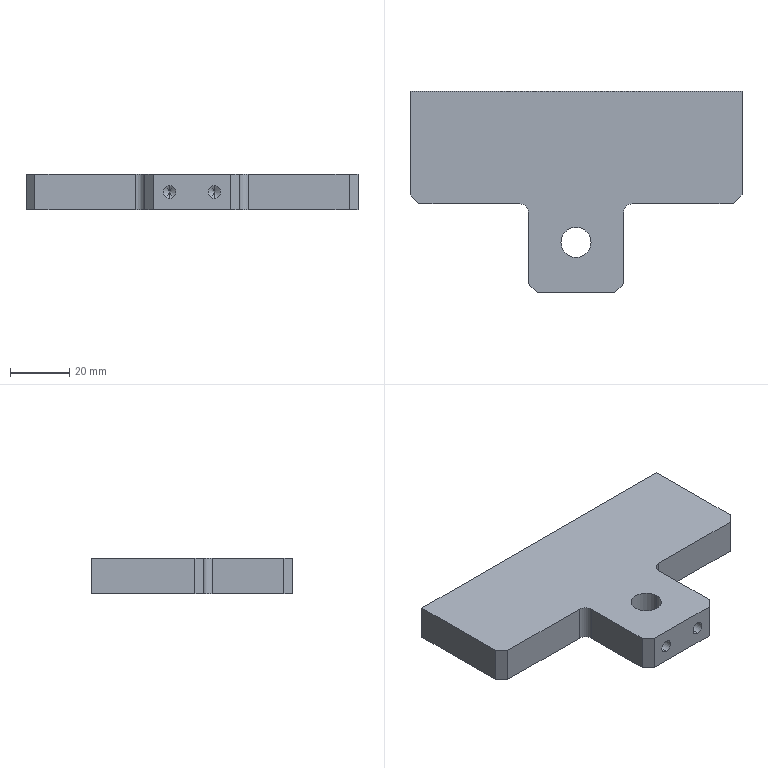Part | SolidWorks | features HoleWzd 3, Chamfer 1, Cut 1, Extrusion 1, Fillet 1, MirrorPattern 1 | 1 solid | 38 faces | box 112 x 68 x 12 mm | volume 60173 mm3 | cylinder 14 | plane 14 | cone 10 | commonest cylinder face diameters 5 x6 4.2 x4 6 x2 10.2 x2
STEP:
#1=CARTESIAN_POINT('',(63.5,12.4,8.1));
#2=VERTEX_POINT('',#1);
#3=CARTESIAN_POINT('',(63.5,12.4,3.9));
#4=VERTEX_POINT('',#3);
#5=CARTESIAN_POINT('',(63.5,12.4,6.));
#6=DIRECTION('',(0.,-1.,0.));
#7=DIRECTION('',(0.,0.,-1.));
#8=AXIS2_PLACEMENT_3D('',#5,#6,#7);
#9=CIRCLE('',#8,2.1);
#10=EDGE_CURVE('',#2,#4,#9,.T.);
#11=ORIENTED_EDGE('',*,*,#10,.F.);
#12=CARTESIAN_POINT('',(63.5,0.,8.1));
#13=VERTEX_POINT('',#12);
#14=CARTESIAN_POINT('',(63.5,0.,8.1));
#15=DIRECTION('',(0.,-1.,0.));
#16=VECTOR('',#15,1000.);
#17=LINE('',#14,#16);
#18=EDGE_CURVE('',#2,#13,#17,.T.);
#19=ORIENTED_EDGE('',*,*,#18,.T.);
#20=CARTESIAN_POINT('',(63.5,0.,3.9));
#21=VERTEX_POINT('',#20);
#22=CARTESIAN_POINT('',(63.5,0.,6.));
#23=DIRECTION('',(0.,-1.,0.));
#24=DIRECTION('',(0.,0.,-1.));
#25=AXIS2_PLACEMENT_3D('',#22,#23,#24);
#26=CIRCLE('',#25,2.1);
#27=EDGE_CURVE('',#13,#21,#26,.T.);
#28=ORIENTED_EDGE('',*,*,#27,.T.);
#29=CARTESIAN_POINT('',(63.5,0.,3.9));
#30=DIRECTION('',(0.,-1.,0.));
#31=VECTOR('',#30,1000.);
#32=LINE('',#29,#31);
#33=EDGE_CURVE('',#4,#21,#32,.T.);
#34=ORIENTED_EDGE('',*,*,#33,.F.);
#35=EDGE_LOOP('',(#11,#19,#28,#34));
#36=FACE_OUTER_BOUND('',#35,.T.);
#37=CARTESIAN_POINT('',(63.5,0.,6.));
#38=DIRECTION('',(0.,-1.,0.));
#39=DIRECTION('',(0.,0.,-1.));
#40=AXIS2_PLACEMENT_3D('',#37,#38,#39);
#41=CYLINDRICAL_SURFACE('',#40,2.1);
#42=ADVANCED_FACE('',(#36),#41,.F.);
#43=CARTESIAN_POINT('',(63.5,13.662,6.));
#44=VERTEX_POINT('',#43);
#45=CARTESIAN_POINT('',(63.5,12.4,3.9));
#46=DIRECTION('',(0.,-0.515,-0.8572));
#47=VECTOR('',#46,1000.);
#48=LINE('',#45,#47);
#49=EDGE_CURVE('',#44,#4,#48,.T.);
#50=ORIENTED_EDGE('',*,*,#49,.F.);
#51=CARTESIAN_POINT('',(63.5,12.4,8.1));
#52=DIRECTION('',(0.,-0.515,0.8572));
#53=VECTOR('',#52,1000.);
#54=LINE('',#51,#53);
#55=EDGE_CURVE('',#44,#2,#54,.T.);
#56=ORIENTED_EDGE('',*,*,#55,.T.);
#57=ORIENTED_EDGE('',*,*,#10,.T.);
#58=EDGE_LOOP('',(#50,#56,#57));
#59=FACE_OUTER_BOUND('',#58,.T.);
#60=CARTESIAN_POINT('',(63.5,12.4,6.));
#61=DIRECTION('',(0.,-1.,0.));
#62=DIRECTION('',(0.,0.,-1.));
#63=AXIS2_PLACEMENT_3D('',#60,#61,#62);
#64=CONICAL_SURFACE('',#63,2.1,1.03);
#65=ADVANCED_FACE('',(#59),#64,.F.);
#66=CARTESIAN_POINT('',(48.5,12.4,8.1));
#67=VERTEX_POINT('',#66);
#68=CARTESIAN_POINT('',(48.5,12.4,3.9));
#69=VERTEX_POINT('',#68);
#70=CARTESIAN_POINT('',(48.5,12.4,6.));
#71=DIRECTION('',(0.,-1.,0.));
#72=DIRECTION('',(0.,0.,-1.));
#73=AXIS2_PLACEMENT_3D('',#70,#71,#72);
#74=CIRCLE('',#73,2.1);
#75=EDGE_CURVE('',#67,#69,#74,.T.);
#76=ORIENTED_EDGE('',*,*,#75,.F.);
#77=CARTESIAN_POINT('',(48.5,0.,8.1));
#78=VERTEX_POINT('',#77);
#79=CARTESIAN_POINT('',(48.5,0.,8.1));
#80=DIRECTION('',(0.,-1.,0.));
#81=VECTOR('',#80,1000.);
#82=LINE('',#79,#81);
#83=EDGE_CURVE('',#67,#78,#82,.T.);
#84=ORIENTED_EDGE('',*,*,#83,.T.);
#85=CARTESIAN_POINT('',(48.5,0.,3.9));
#86=VERTEX_POINT('',#85);
#87=CARTESIAN_POINT('',(48.5,0.,6.));
#88=DIRECTION('',(0.,-1.,0.));
#89=DIRECTION('',(0.,0.,-1.));
#90=AXIS2_PLACEMENT_3D('',#87,#88,#89);
#91=CIRCLE('',#90,2.1);
#92=EDGE_CURVE('',#78,#86,#91,.T.);
#93=ORIENTED_EDGE('',*,*,#92,.T.);
#94=CARTESIAN_POINT('',(48.5,0.,3.9));
#95=DIRECTION('',(0.,-1.,0.));
#96=VECTOR('',#95,1000.);
#97=LINE('',#94,#96);
#98=EDGE_CURVE('',#69,#86,#97,.T.);
#99=ORIENTED_EDGE('',*,*,#98,.F.);
#100=EDGE_LOOP('',(#76,#84,#93,#99));
#101=FACE_OUTER_BOUND('',#100,.T.);
#102=CARTESIAN_POINT('',(48.5,0.,6.));
#103=DIRECTION('',(0.,-1.,0.));
#104=DIRECTION('',(0.,0.,-1.));
#105=AXIS2_PLACEMENT_3D('',#102,#103,#104);
#106=CYLINDRICAL_SURFACE('',#105,2.1);
#107=ADVANCED_FACE('',(#101),#106,.F.);
#108=CARTESIAN_POINT('',(48.5,13.662,6.));
#109=VERTEX_POINT('',#108);
#110=CARTESIAN_POINT('',(48.5,12.4,3.9));
#111=DIRECTION('',(0.,-0.515,-0.8572));
#112=VECTOR('',#111,1000.);
#113=LINE('',#110,#112);
#114=EDGE_CURVE('',#109,#69,#113,.T.);
#115=ORIENTED_EDGE('',*,*,#114,.F.);
#116=CARTESIAN_POINT('',(48.5,12.4,8.1));
#117=DIRECTION('',(0.,-0.515,0.8572));
#118=VECTOR('',#117,1000.);
#119=LINE('',#116,#118);
#120=EDGE_CURVE('',#109,#67,#119,.T.);
#121=ORIENTED_EDGE('',*,*,#120,.T.);
#122=ORIENTED_EDGE('',*,*,#75,.T.);
#123=EDGE_LOOP('',(#115,#121,#122));
#124=FACE_OUTER_BOUND('',#123,.T.);
#125=CARTESIAN_POINT('',(48.5,12.4,6.));
#126=DIRECTION('',(0.,-1.,0.));
#127=DIRECTION('',(0.,0.,-1.));
#128=AXIS2_PLACEMENT_3D('',#125,#126,#127);
#129=CONICAL_SURFACE('',#128,2.1,1.03);
#130=ADVANCED_FACE('',(#124),#129,.F.);
#131=CARTESIAN_POINT('',(101.,53.,3.5));
#132=VERTEX_POINT('',#131);
#133=CARTESIAN_POINT('',(101.,53.,8.5));
#134=VERTEX_POINT('',#133);
#135=CARTESIAN_POINT('',(101.,53.,6.));
#136=DIRECTION('',(0.,1.,0.));
#137=DIRECTION('',(0.,0.,1.));
#138=AXIS2_PLACEMENT_3D('',#135,#136,#137);
#139=CIRCLE('',#138,2.5);
#140=EDGE_CURVE('',#132,#134,#139,.T.);
#141=ORIENTED_EDGE('',*,*,#140,.F.);
#142=CARTESIAN_POINT('',(101.,68.,3.5));
#143=VERTEX_POINT('',#142);
#144=CARTESIAN_POINT('',(101.,68.,3.5));
#145=DIRECTION('',(0.,1.,0.));
#146=VECTOR('',#145,1000.);
#147=LINE('',#144,#146);
#148=EDGE_CURVE('',#132,#143,#147,.T.);
#149=ORIENTED_EDGE('',*,*,#148,.T.);
#150=CARTESIAN_POINT('',(101.,68.,8.5));
#151=VERTEX_POINT('',#150);
#152=CARTESIAN_POINT('',(101.,68.,6.));
#153=DIRECTION('',(0.,1.,0.));
#154=DIRECTION('',(0.,0.,1.));
#155=AXIS2_PLACEMENT_3D('',#152,#153,#154);
#156=CIRCLE('',#155,2.5);
#157=EDGE_CURVE('',#143,#151,#156,.T.);
#158=ORIENTED_EDGE('',*,*,#157,.T.);
#159=CARTESIAN_POINT('',(101.,68.,8.5));
#160=DIRECTION('',(0.,1.,0.));
#161=VECTOR('',#160,1000.);
#162=LINE('',#159,#161);
#163=EDGE_CURVE('',#134,#151,#162,.T.);
#164=ORIENTED_EDGE('',*,*,#163,.F.);
#165=EDGE_LOOP('',(#141,#149,#158,#164));
#166=FACE_OUTER_BOUND('',#165,.T.);
#167=CARTESIAN_POINT('',(101.,68.,6.));
#168=DIRECTION('',(0.,1.,0.));
#169=DIRECTION('',(0.,0.,1.));
#170=AXIS2_PLACEMENT_3D('',#167,#168,#169);
#171=CYLINDRICAL_SURFACE('',#170,2.5);
#172=ADVANCED_FACE('',(#166),#171,.F.);
#173=CARTESIAN_POINT('',(101.,51.498,6.));
#174=VERTEX_POINT('',#173);
#175=CARTESIAN_POINT('',(101.,53.,8.5));
#176=DIRECTION('',(0.,0.515,0.8572));
#177=VECTOR('',#176,1000.);
#178=LINE('',#175,#177);
#179=EDGE_CURVE('',#174,#134,#178,.T.);
#180=ORIENTED_EDGE('',*,*,#179,.F.);
#181=CARTESIAN_POINT('',(101.,53.,3.5));
#182=DIRECTION('',(0.,0.515,-0.8572));
#183=VECTOR('',#182,1000.);
#184=LINE('',#181,#183);
#185=EDGE_CURVE('',#174,#132,#184,.T.);
#186=ORIENTED_EDGE('',*,*,#185,.T.);
#187=ORIENTED_EDGE('',*,*,#140,.T.);
#188=EDGE_LOOP('',(#180,#186,#187));
#189=FACE_OUTER_BOUND('',#188,.T.);
#190=CARTESIAN_POINT('',(101.,53.,6.));
#191=DIRECTION('',(0.,1.,0.));
#192=DIRECTION('',(0.,0.,1.));
#193=AXIS2_PLACEMENT_3D('',#190,#191,#192);
#194=CONICAL_SURFACE('',#193,2.5,1.03);
#195=ADVANCED_FACE('',(#189),#194,.F.);
#196=CARTESIAN_POINT('',(56.,53.,3.5));
#197=VERTEX_POINT('',#196);
#198=CARTESIAN_POINT('',(56.,53.,8.5));
#199=VERTEX_POINT('',#198);
#200=CARTESIAN_POINT('',(56.,53.,6.));
#201=DIRECTION('',(0.,1.,0.));
#202=DIRECTION('',(0.,0.,1.));
#203=AXIS2_PLACEMENT_3D('',#200,#201,#202);
#204=CIRCLE('',#203,2.5);
#205=EDGE_CURVE('',#197,#199,#204,.T.);
#206=ORIENTED_EDGE('',*,*,#205,.F.);
#207=CARTESIAN_POINT('',(56.,68.,3.5));
#208=VERTEX_POINT('',#207);
#209=CARTESIAN_POINT('',(56.,68.,3.5));
#210=DIRECTION('',(0.,1.,0.));
#211=VECTOR('',#210,1000.);
#212=LINE('',#209,#211);
#213=EDGE_CURVE('',#197,#208,#212,.T.);
#214=ORIENTED_EDGE('',*,*,#213,.T.);
#215=CARTESIAN_POINT('',(56.,68.,8.5));
#216=VERTEX_POINT('',#215);
#217=CARTESIAN_POINT('',(56.,68.,6.));
#218=DIRECTION('',(0.,1.,0.));
#219=DIRECTION('',(0.,0.,1.));
#220=AXIS2_PLACEMENT_3D('',#217,#218,#219);
#221=CIRCLE('',#220,2.5);
#222=EDGE_CURVE('',#208,#216,#221,.T.);
#223=ORIENTED_EDGE('',*,*,#222,.T.);
#224=CARTESIAN_POINT('',(56.,68.,8.5));
#225=DIRECTION('',(0.,1.,0.));
#226=VECTOR('',#225,1000.);
#227=LINE('',#224,#226);
#228=EDGE_CURVE('',#199,#216,#227,.T.);
#229=ORIENTED_EDGE('',*,*,#228,.F.);
#230=EDGE_LOOP('',(#206,#214,#223,#229));
#231=FACE_OUTER_BOUND('',#230,.T.);
#232=CARTESIAN_POINT('',(56.,68.,6.));
#233=DIRECTION('',(0.,1.,0.));
#234=DIRECTION('',(0.,0.,1.));
#235=AXIS2_PLACEMENT_3D('',#232,#233,#234);
#236=CYLINDRICAL_SURFACE('',#235,2.5);
#237=ADVANCED_FACE('',(#231),#236,.F.);
#238=CARTESIAN_POINT('',(56.,51.498,6.));
#239=VERTEX_POINT('',#238);
#240=CARTESIAN_POINT('',(56.,53.,8.5));
#241=DIRECTION('',(0.,0.515,0.8572));
#242=VECTOR('',#241,1000.);
#243=LINE('',#240,#242);
#244=EDGE_CURVE('',#239,#199,#243,.T.);
#245=ORIENTED_EDGE('',*,*,#244,.F.);
#246=CARTESIAN_POINT('',(56.,53.,3.5));
#247=DIRECTION('',(0.,0.515,-0.8572));
#248=VECTOR('',#247,1000.);
#249=LINE('',#246,#248);
#250=EDGE_CURVE('',#239,#197,#249,.T.);
#251=ORIENTED_EDGE('',*,*,#250,.T.);
#252=ORIENTED_EDGE('',*,*,#205,.T.);
#253=EDGE_LOOP('',(#245,#251,#252));
#254=FACE_OUTER_BOUND('',#253,.T.);
#255=CARTESIAN_POINT('',(56.,53.,6.));
#256=DIRECTION('',(0.,1.,0.));
#257=DIRECTION('',(0.,0.,1.));
#258=AXIS2_PLACEMENT_3D('',#255,#256,#257);
#259=CONICAL_SURFACE('',#258,2.5,1.03);
#260=ADVANCED_FACE('',(#254),#259,.F.);
#261=CARTESIAN_POINT('',(11.,53.,3.5));
#262=VERTEX_POINT('',#261);
#263=CARTESIAN_POINT('',(11.,53.,8.5));
#264=VERTEX_POINT('',#263);
#265=CARTESIAN_POINT('',(11.,53.,6.));
#266=DIRECTION('',(0.,1.,0.));
#267=DIRECTION('',(0.,0.,1.));
#268=AXIS2_PLACEMENT_3D('',#265,#266,#267);
#269=CIRCLE('',#268,2.5);
#270=EDGE_CURVE('',#262,#264,#269,.T.);
#271=ORIENTED_EDGE('',*,*,#270,.F.);
#272=CARTESIAN_POINT('',(11.,68.,3.5));
#273=VERTEX_POINT('',#272);
#274=CARTESIAN_POINT('',(11.,68.,3.5));
#275=DIRECTION('',(0.,1.,0.));
#276=VECTOR('',#275,1000.);
#277=LINE('',#274,#276);
#278=EDGE_CURVE('',#262,#273,#277,.T.);
#279=ORIENTED_EDGE('',*,*,#278,.T.);
#280=CARTESIAN_POINT('',(11.,68.,8.5));
#281=VERTEX_POINT('',#280);
#282=CARTESIAN_POINT('',(11.,68.,6.));
#283=DIRECTION('',(0.,1.,0.));
#284=DIRECTION('',(0.,0.,1.));
#285=AXIS2_PLACEMENT_3D('',#282,#283,#284);
#286=CIRCLE('',#285,2.5);
#287=EDGE_CURVE('',#273,#281,#286,.T.);
#288=ORIENTED_EDGE('',*,*,#287,.T.);
#289=CARTESIAN_POINT('',(11.,68.,8.5));
#290=DIRECTION('',(0.,1.,0.));
#291=VECTOR('',#290,1000.);
#292=LINE('',#289,#291);
#293=EDGE_CURVE('',#264,#281,#292,.T.);
#294=ORIENTED_EDGE('',*,*,#293,.F.);
#295=EDGE_LOOP('',(#271,#279,#288,#294));
#296=FACE_OUTER_BOUND('',#295,.T.);
#297=CARTESIAN_POINT('',(11.,68.,6.));
#298=DIRECTION('',(0.,1.,0.));
#299=DIRECTION('',(0.,0.,1.));
#300=AXIS2_PLACEMENT_3D('',#297,#298,#299);
#301=CYLINDRICAL_SURFACE('',#300,2.5);
#302=ADVANCED_FACE('',(#296),#301,.F.);
#303=CARTESIAN_POINT('',(11.,51.498,6.));
#304=VERTEX_POINT('',#303);
#305=CARTESIAN_POINT('',(11.,53.,8.5));
#306=DIRECTION('',(0.,0.515,0.8572));
#307=VECTOR('',#306,1000.);
#308=LINE('',#305,#307);
#309=EDGE_CURVE('',#304,#264,#308,.T.);
#310=ORIENTED_EDGE('',*,*,#309,.F.);
#311=CARTESIAN_POINT('',(11.,53.,3.5));
#312=DIRECTION('',(0.,0.515,-0.8572));
#313=VECTOR('',#312,1000.);
#314=LINE('',#311,#313);
#315=EDGE_CURVE('',#304,#262,#314,.T.);
#316=ORIENTED_EDGE('',*,*,#315,.T.);
#317=ORIENTED_EDGE('',*,*,#270,.T.);
#318=EDGE_LOOP('',(#310,#316,#317));
#319=FACE_OUTER_BOUND('',#318,.T.);
#320=CARTESIAN_POINT('',(11.,53.,6.));
#321=DIRECTION('',(0.,1.,0.));
#322=DIRECTION('',(0.,0.,1.));
#323=AXIS2_PLACEMENT_3D('',#320,#321,#322);
#324=CONICAL_SURFACE('',#323,2.5,1.03);
#325=ADVANCED_FACE('',(#319),#324,.F.);
#326=CARTESIAN_POINT('',(50.9,17.,0.));
#327=VERTEX_POINT('',#326);
#328=CARTESIAN_POINT('',(61.1,17.,0.));
#329=VERTEX_POINT('',#328);
#330=CARTESIAN_POINT('',(56.,17.,0.));
#331=DIRECTION('',(0.,0.,1.));
#332=DIRECTION('',(1.,0.,0.));
#333=AXIS2_PLACEMENT_3D('',#330,#331,#332);
#334=CIRCLE('',#333,5.1);
#335=EDGE_CURVE('',#327,#329,#334,.T.);
#336=ORIENTED_EDGE('',*,*,#335,.F.);
#337=CARTESIAN_POINT('',(50.9,17.,12.));
#338=VERTEX_POINT('',#337);
#339=CARTESIAN_POINT('',(50.9,17.,12.));
#340=DIRECTION('',(0.,0.,1.));
#341=VECTOR('',#340,1000.);
#342=LINE('',#339,#341);
#343=EDGE_CURVE('',#327,#338,#342,.T.);
#344=ORIENTED_EDGE('',*,*,#343,.T.);
#345=CARTESIAN_POINT('',(61.1,17.,12.));
#346=VERTEX_POINT('',#345);
#347=CARTESIAN_POINT('',(56.,17.,12.));
#348=DIRECTION('',(0.,0.,1.));
#349=DIRECTION('',(1.,0.,0.));
#350=AXIS2_PLACEMENT_3D('',#347,#348,#349);
#351=CIRCLE('',#350,5.1);
#352=EDGE_CURVE('',#338,#346,#351,.T.);
#353=ORIENTED_EDGE('',*,*,#352,.T.);
#354=CARTESIAN_POINT('',(61.1,17.,12.));
#355=DIRECTION('',(0.,0.,1.));
#356=VECTOR('',#355,1000.);
#357=LINE('',#354,#356);
#358=EDGE_CURVE('',#329,#346,#357,.T.);
#359=ORIENTED_EDGE('',*,*,#358,.F.);
#360=EDGE_LOOP('',(#336,#344,#353,#359));
#361=FACE_OUTER_BOUND('',#360,.T.);
#362=CARTESIAN_POINT('',(56.,17.,12.));
#363=DIRECTION('',(0.,0.,1.));
#364=DIRECTION('',(1.,0.,0.));
#365=AXIS2_PLACEMENT_3D('',#362,#363,#364);
#366=CYLINDRICAL_SURFACE('',#365,5.1);
#367=ADVANCED_FACE('',(#361),#366,.F.);
#368=CARTESIAN_POINT('',(63.5,0.,6.));
#369=DIRECTION('',(0.,-1.,0.));
#370=DIRECTION('',(0.,0.,-1.));
#371=AXIS2_PLACEMENT_3D('',#368,#369,#370);
#372=CIRCLE('',#371,2.1);
#373=EDGE_CURVE('',#21,#13,#372,.T.);
#374=ORIENTED_EDGE('',*,*,#373,.F.);
#375=ORIENTED_EDGE('',*,*,#27,.F.);
#376=EDGE_LOOP('',(#374,#375));
#377=FACE_BOUND('',#376,.T.);
#378=CARTESIAN_POINT('',(48.5,0.,6.));
#379=DIRECTION('',(0.,-1.,0.));
#380=DIRECTION('',(0.,0.,-1.));
#381=AXIS2_PLACEMENT_3D('',#378,#379,#380);
#382=CIRCLE('',#381,2.1);
#383=EDGE_CURVE('',#86,#78,#382,.T.);
#384=ORIENTED_EDGE('',*,*,#383,.F.);
#385=ORIENTED_EDGE('',*,*,#92,.F.);
#386=EDGE_LOOP('',(#384,#385));
#387=FACE_BOUND('',#386,.T.);
#388=CARTESIAN_POINT('',(43.,0.,0.));
#389=VERTEX_POINT('',#388);
#390=CARTESIAN_POINT('',(69.,0.,0.));
#391=VERTEX_POINT('',#390);
#392=CARTESIAN_POINT('',(0.,0.,0.));
#393=DIRECTION('',(1.,0.,0.));
#394=VECTOR('',#393,1000.);
#395=LINE('',#392,#394);
#396=EDGE_CURVE('',#389,#391,#395,.T.);
#397=ORIENTED_EDGE('',*,*,#396,.T.);
#398=CARTESIAN_POINT('',(69.,0.,12.));
#399=VERTEX_POINT('',#398);
#400=CARTESIAN_POINT('',(69.,0.,12.));
#401=DIRECTION('',(0.,0.,1.));
#402=VECTOR('',#401,1000.);
#403=LINE('',#400,#402);
#404=EDGE_CURVE('',#391,#399,#403,.T.);
#405=ORIENTED_EDGE('',*,*,#404,.T.);
#406=CARTESIAN_POINT('',(43.,0.,12.));
#407=VERTEX_POINT('',#406);
#408=CARTESIAN_POINT('',(0.,0.,12.));
#409=DIRECTION('',(1.,0.,0.));
#410=VECTOR('',#409,1000.);
#411=LINE('',#408,#410);
#412=EDGE_CURVE('',#407,#399,#411,.T.);
#413=ORIENTED_EDGE('',*,*,#412,.F.);
#414=CARTESIAN_POINT('',(43.,0.,12.));
#415=DIRECTION('',(0.,0.,-1.));
#416=VECTOR('',#415,1000.);
#417=LINE('',#414,#416);
#418=EDGE_CURVE('',#407,#389,#417,.T.);
#419=ORIENTED_EDGE('',*,*,#418,.T.);
#420=EDGE_LOOP('',(#397,#405,#413,#419));
#421=FACE_OUTER_BOUND('',#420,.T.);
#422=CARTESIAN_POINT('',(0.,0.,12.));
#423=DIRECTION('',(0.,1.,0.));
#424=DIRECTION('',(0.,0.,1.));
#425=AXIS2_PLACEMENT_3D('',#422,#423,#424);
#426=PLANE('',#425);
#427=ADVANCED_FACE('',(#377,#387,#421),#426,.F.);
#428=CARTESIAN_POINT('',(112.,33.,12.));
#429=VERTEX_POINT('',#428);
#430=CARTESIAN_POINT('',(112.,68.,12.));
#431=VERTEX_POINT('',#430);
#432=CARTESIAN_POINT('',(112.,0.,12.));
#433=DIRECTION('',(0.,1.,0.));
#434=VECTOR('',#433,1000.);
#435=LINE('',#432,#434);
#436=EDGE_CURVE('',#429,#431,#435,.T.);
#437=ORIENTED_EDGE('',*,*,#436,.F.);
#438=CARTESIAN_POINT('',(112.,33.,0.));
#439=VERTEX_POINT('',#438);
#440=CARTESIAN_POINT('',(112.,33.,0.));
#441=DIRECTION('',(0.,0.,-1.));
#442=VECTOR('',#441,1000.);
#443=LINE('',#440,#442);
#444=EDGE_CURVE('',#429,#439,#443,.T.);
#445=ORIENTED_EDGE('',*,*,#444,.T.);
#446=CARTESIAN_POINT('',(112.,68.,0.));
#447=VERTEX_POINT('',#446);
#448=CARTESIAN_POINT('',(112.,0.,0.));
#449=DIRECTION('',(0.,1.,0.));
#450=VECTOR('',#449,1000.);
#451=LINE('',#448,#450);
#452=EDGE_CURVE('',#439,#447,#451,.T.);
#453=ORIENTED_EDGE('',*,*,#452,.T.);
#454=CARTESIAN_POINT('',(112.,68.,12.));
#455=DIRECTION('',(0.,0.,-1.));
#456=VECTOR('',#455,1000.);
#457=LINE('',#454,#456);
#458=EDGE_CURVE('',#431,#447,#457,.T.);
#459=ORIENTED_EDGE('',*,*,#458,.F.);
#460=EDGE_LOOP('',(#437,#445,#453,#459));
#461=FACE_OUTER_BOUND('',#460,.T.);
#462=CARTESIAN_POINT('',(112.,0.,12.));
#463=DIRECTION('',(-1.,0.,0.));
#464=DIRECTION('',(0.,-1.,0.));
#465=AXIS2_PLACEMENT_3D('',#462,#463,#464);
#466=PLANE('',#465);
#467=ADVANCED_FACE('',(#461),#466,.F.);
#468=CARTESIAN_POINT('',(56.,17.,12.));
#469=DIRECTION('',(0.,0.,1.));
#470=DIRECTION('',(1.,0.,0.));
#471=AXIS2_PLACEMENT_3D('',#468,#469,#470);
#472=CIRCLE('',#471,5.1);
#473=EDGE_CURVE('',#346,#338,#472,.T.);
#474=ORIENTED_EDGE('',*,*,#473,.F.);
#475=ORIENTED_EDGE('',*,*,#352,.F.);
#476=EDGE_LOOP('',(#474,#475));
#477=FACE_BOUND('',#476,.T.);
#478=ORIENTED_EDGE('',*,*,#412,.T.);
#479=CARTESIAN_POINT('',(72.,3.,12.));
#480=VERTEX_POINT('',#479);
#481=CARTESIAN_POINT('',(69.,0.,12.));
#482=DIRECTION('',(0.7071,0.7071,0.));
#483=VECTOR('',#482,1000.);
#484=LINE('',#481,#483);
#485=EDGE_CURVE('',#399,#480,#484,.T.);
#486=ORIENTED_EDGE('',*,*,#485,.T.);
#487=CARTESIAN_POINT('',(72.,27.,12.));
#488=VERTEX_POINT('',#487);
#489=CARTESIAN_POINT('',(72.,0.,12.));
#490=DIRECTION('',(0.,1.,0.));
#491=VECTOR('',#490,1000.);
#492=LINE('',#489,#491);
#493=EDGE_CURVE('',#480,#488,#492,.T.);
#494=ORIENTED_EDGE('',*,*,#493,.T.);
#495=CARTESIAN_POINT('',(75.,30.,12.));
#496=VERTEX_POINT('',#495);
#497=CARTESIAN_POINT('',(75.,27.,12.));
#498=DIRECTION('',(0.,0.,-1.));
#499=DIRECTION('',(-1.,0.,0.));
#500=AXIS2_PLACEMENT_3D('',#497,#498,#499);
#501=CIRCLE('',#500,3.);
#502=EDGE_CURVE('',#488,#496,#501,.T.);
#503=ORIENTED_EDGE('',*,*,#502,.T.);
#504=CARTESIAN_POINT('',(109.,30.,12.));
#505=VERTEX_POINT('',#504);
#506=CARTESIAN_POINT('',(112.,30.,12.));
#507=DIRECTION('',(1.,0.,0.));
#508=VECTOR('',#507,1000.);
#509=LINE('',#506,#508);
#510=EDGE_CURVE('',#496,#505,#509,.T.);
#511=ORIENTED_EDGE('',*,*,#510,.T.);
#512=CARTESIAN_POINT('',(109.,30.,12.));
#513=DIRECTION('',(0.7071,0.7071,0.));
#514=VECTOR('',#513,1000.);
#515=LINE('',#512,#514);
#516=EDGE_CURVE('',#505,#429,#515,.T.);
#517=ORIENTED_EDGE('',*,*,#516,.T.);
#518=ORIENTED_EDGE('',*,*,#436,.T.);
#519=CARTESIAN_POINT('',(0.,68.,12.));
#520=VERTEX_POINT('',#519);
#521=CARTESIAN_POINT('',(0.,68.,12.));
#522=DIRECTION('',(-1.,0.,0.));
#523=VECTOR('',#522,1000.);
#524=LINE('',#521,#523);
#525=EDGE_CURVE('',#431,#520,#524,.T.);
#526=ORIENTED_EDGE('',*,*,#525,.T.);
#527=CARTESIAN_POINT('',(0.,33.,12.));
#528=VERTEX_POINT('',#527);
#529=CARTESIAN_POINT('',(0.,0.,12.));
#530=DIRECTION('',(0.,-1.,0.));
#531=VECTOR('',#530,1000.);
#532=LINE('',#529,#531);
#533=EDGE_CURVE('',#520,#528,#532,.T.);
#534=ORIENTED_EDGE('',*,*,#533,.T.);
#535=CARTESIAN_POINT('',(3.,30.,12.));
#536=VERTEX_POINT('',#535);
#537=CARTESIAN_POINT('',(0.,33.,12.));
#538=DIRECTION('',(0.7071,-0.7071,0.));
#539=VECTOR('',#538,1000.);
#540=LINE('',#537,#539);
#541=EDGE_CURVE('',#528,#536,#540,.T.);
#542=ORIENTED_EDGE('',*,*,#541,.T.);
#543=CARTESIAN_POINT('',(37.,30.,12.));
#544=VERTEX_POINT('',#543);
#545=CARTESIAN_POINT('',(0.,30.,12.));
#546=DIRECTION('',(-1.,0.,0.));
#547=VECTOR('',#546,1000.);
#548=LINE('',#545,#547);
#549=EDGE_CURVE('',#544,#536,#548,.T.);
#550=ORIENTED_EDGE('',*,*,#549,.F.);
#551=CARTESIAN_POINT('',(40.,27.,12.));
#552=VERTEX_POINT('',#551);
#553=CARTESIAN_POINT('',(37.,27.,12.));
#554=DIRECTION('',(0.,0.,-1.));
#555=DIRECTION('',(-1.,0.,0.));
#556=AXIS2_PLACEMENT_3D('',#553,#554,#555);
#557=CIRCLE('',#556,3.);
#558=EDGE_CURVE('',#544,#552,#557,.T.);
#559=ORIENTED_EDGE('',*,*,#558,.T.);
#560=CARTESIAN_POINT('',(40.,3.,12.));
#561=VERTEX_POINT('',#560);
#562=CARTESIAN_POINT('',(40.,0.,12.));
#563=DIRECTION('',(0.,1.,0.));
#564=VECTOR('',#563,1000.);
#565=LINE('',#562,#564);
#566=EDGE_CURVE('',#561,#552,#565,.T.);
#567=ORIENTED_EDGE('',*,*,#566,.F.);
#568=CARTESIAN_POINT('',(40.,3.,12.));
#569=DIRECTION('',(0.7071,-0.7071,0.));
#570=VECTOR('',#569,1000.);
#571=LINE('',#568,#570);
#572=EDGE_CURVE('',#561,#407,#571,.T.);
#573=ORIENTED_EDGE('',*,*,#572,.T.);
#574=EDGE_LOOP('',(#478,#486,#494,#503,#511,#517,#518,#526,#534,#542,#550,#559,#567,#573));
#575=FACE_OUTER_BOUND('',#574,.T.);
#576=CARTESIAN_POINT('',(0.,0.,12.));
#577=DIRECTION('',(0.,0.,-1.));
#578=DIRECTION('',(-1.,0.,0.));
#579=AXIS2_PLACEMENT_3D('',#576,#577,#578);
#580=PLANE('',#579);
#581=ADVANCED_FACE('',(#477,#575),#580,.F.);
#582=CARTESIAN_POINT('',(56.,17.,0.));
#583=DIRECTION('',(0.,0.,1.));
#584=DIRECTION('',(1.,0.,0.));
#585=AXIS2_PLACEMENT_3D('',#582,#583,#584);
#586=CIRCLE('',#585,5.1);
#587=EDGE_CURVE('',#329,#327,#586,.T.);
#588=ORIENTED_EDGE('',*,*,#587,.T.);
#589=ORIENTED_EDGE('',*,*,#335,.T.);
#590=EDGE_LOOP('',(#588,#589));
#591=FACE_BOUND('',#590,.T.);
#592=CARTESIAN_POINT('',(72.,3.,0.));
#593=VERTEX_POINT('',#592);
#594=CARTESIAN_POINT('',(72.,27.,0.));
#595=VERTEX_POINT('',#594);
#596=CARTESIAN_POINT('',(72.,0.,0.));
#597=DIRECTION('',(0.,1.,0.));
#598=VECTOR('',#597,1000.);
#599=LINE('',#596,#598);
#600=EDGE_CURVE('',#593,#595,#599,.T.);
#601=ORIENTED_EDGE('',*,*,#600,.F.);
#602=CARTESIAN_POINT('',(34.5,-34.5,0.));
#603=DIRECTION('',(-0.7071,-0.7071,0.));
#604=VECTOR('',#603,1000.);
#605=LINE('',#602,#604);
#606=EDGE_CURVE('',#593,#391,#605,.T.);
#607=ORIENTED_EDGE('',*,*,#606,.T.);
#608=ORIENTED_EDGE('',*,*,#396,.F.);
#609=CARTESIAN_POINT('',(40.,3.,0.));
#610=VERTEX_POINT('',#609);
#611=CARTESIAN_POINT('',(21.5,21.5,0.));
#612=DIRECTION('',(-0.7071,0.7071,0.));
#613=VECTOR('',#612,1000.);
#614=LINE('',#611,#613);
#615=EDGE_CURVE('',#389,#610,#614,.T.);
#616=ORIENTED_EDGE('',*,*,#615,.T.);
#617=CARTESIAN_POINT('',(40.,27.,0.));
#618=VERTEX_POINT('',#617);
#619=CARTESIAN_POINT('',(40.,0.,0.));
#620=DIRECTION('',(0.,1.,0.));
#621=VECTOR('',#620,1000.);
#622=LINE('',#619,#621);
#623=EDGE_CURVE('',#610,#618,#622,.T.);
#624=ORIENTED_EDGE('',*,*,#623,.T.);
#625=CARTESIAN_POINT('',(37.,30.,0.));
#626=VERTEX_POINT('',#625);
#627=CARTESIAN_POINT('',(37.,27.,0.));
#628=DIRECTION('',(0.,0.,1.));
#629=DIRECTION('',(-1.,0.,0.));
#630=AXIS2_PLACEMENT_3D('',#627,#628,#629);
#631=CIRCLE('',#630,3.);
#632=EDGE_CURVE('',#618,#626,#631,.T.);
#633=ORIENTED_EDGE('',*,*,#632,.T.);
#634=CARTESIAN_POINT('',(3.,30.,0.));
#635=VERTEX_POINT('',#634);
#636=CARTESIAN_POINT('',(0.,30.,0.));
#637=DIRECTION('',(-1.,0.,0.));
#638=VECTOR('',#637,1000.);
#639=LINE('',#636,#638);
#640=EDGE_CURVE('',#626,#635,#639,.T.);
#641=ORIENTED_EDGE('',*,*,#640,.T.);
#642=CARTESIAN_POINT('',(0.,33.,0.));
#643=VERTEX_POINT('',#642);
#644=CARTESIAN_POINT('',(16.5,16.5,0.));
#645=DIRECTION('',(-0.7071,0.7071,0.));
#646=VECTOR('',#645,1000.);
#647=LINE('',#644,#646);
#648=EDGE_CURVE('',#635,#643,#647,.T.);
#649=ORIENTED_EDGE('',*,*,#648,.T.);
#650=CARTESIAN_POINT('',(0.,68.,0.));
#651=VERTEX_POINT('',#650);
#652=CARTESIAN_POINT('',(0.,0.,0.));
#653=DIRECTION('',(0.,-1.,0.));
#654=VECTOR('',#653,1000.);
#655=LINE('',#652,#654);
#656=EDGE_CURVE('',#651,#643,#655,.T.);
#657=ORIENTED_EDGE('',*,*,#656,.F.);
#658=CARTESIAN_POINT('',(0.,68.,0.));
#659=DIRECTION('',(-1.,0.,0.));
#660=VECTOR('',#659,1000.);
#661=LINE('',#658,#660);
#662=EDGE_CURVE('',#447,#651,#661,.T.);
#663=ORIENTED_EDGE('',*,*,#662,.F.);
#664=ORIENTED_EDGE('',*,*,#452,.F.);
#665=CARTESIAN_POINT('',(109.,30.,0.));
#666=VERTEX_POINT('',#665);
#667=CARTESIAN_POINT('',(39.5,-39.5,0.));
#668=DIRECTION('',(-0.7071,-0.7071,0.));
#669=VECTOR('',#668,1000.);
#670=LINE('',#667,#669);
#671=EDGE_CURVE('',#439,#666,#670,.T.);
#672=ORIENTED_EDGE('',*,*,#671,.T.);
#673=CARTESIAN_POINT('',(75.,30.,0.));
#674=VERTEX_POINT('',#673);
#675=CARTESIAN_POINT('',(112.,30.,0.));
#676=DIRECTION('',(1.,0.,0.));
#677=VECTOR('',#676,1000.);
#678=LINE('',#675,#677);
#679=EDGE_CURVE('',#674,#666,#678,.T.);
#680=ORIENTED_EDGE('',*,*,#679,.F.);
#681=CARTESIAN_POINT('',(75.,27.,0.));
#682=DIRECTION('',(0.,0.,1.));
#683=DIRECTION('',(-1.,0.,0.));
#684=AXIS2_PLACEMENT_3D('',#681,#682,#683);
#685=CIRCLE('',#684,3.);
#686=EDGE_CURVE('',#674,#595,#685,.T.);
#687=ORIENTED_EDGE('',*,*,#686,.T.);
#688=EDGE_LOOP('',(#601,#607,#608,#616,#624,#633,#641,#649,#657,#663,#664,#672,#680,#687));
#689=FACE_OUTER_BOUND('',#688,.T.);
#690=CARTESIAN_POINT('',(0.,0.,0.));
#691=DIRECTION('',(0.,0.,-1.));
#692=DIRECTION('',(-1.,0.,0.));
#693=AXIS2_PLACEMENT_3D('',#690,#691,#692);
#694=PLANE('',#693);
#695=ADVANCED_FACE('',(#591,#689),#694,.T.);
#696=ORIENTED_EDGE('',*,*,#656,.T.);
#697=CARTESIAN_POINT('',(0.,33.,12.));
#698=DIRECTION('',(0.,0.,1.));
#699=VECTOR('',#698,1000.);
#700=LINE('',#697,#699);
#701=EDGE_CURVE('',#643,#528,#700,.T.);
#702=ORIENTED_EDGE('',*,*,#701,.T.);
#703=ORIENTED_EDGE('',*,*,#533,.F.);
#704=CARTESIAN_POINT('',(0.,68.,12.));
#705=DIRECTION('',(0.,0.,-1.));
#706=VECTOR('',#705,1000.);
#707=LINE('',#704,#706);
#708=EDGE_CURVE('',#520,#651,#707,.T.);
#709=ORIENTED_EDGE('',*,*,#708,.T.);
#710=EDGE_LOOP('',(#696,#702,#703,#709));
#711=FACE_OUTER_BOUND('',#710,.T.);
#712=CARTESIAN_POINT('',(0.,0.,12.));
#713=DIRECTION('',(1.,0.,0.));
#714=DIRECTION('',(0.,1.,0.));
#715=AXIS2_PLACEMENT_3D('',#712,#713,#714);
#716=PLANE('',#715);
#717=ADVANCED_FACE('',(#711),#716,.F.);
#718=CARTESIAN_POINT('',(101.,68.,6.));
#719=DIRECTION('',(0.,1.,0.));
#720=DIRECTION('',(0.,0.,1.));
#721=AXIS2_PLACEMENT_3D('',#718,#719,#720);
#722=CIRCLE('',#721,2.5);
#723=EDGE_CURVE('',#151,#143,#722,.T.);
#724=ORIENTED_EDGE('',*,*,#723,.F.);
#725=ORIENTED_EDGE('',*,*,#157,.F.);
#726=EDGE_LOOP('',(#724,#725));
#727=FACE_BOUND('',#726,.T.);
#728=CARTESIAN_POINT('',(56.,68.,6.));
#729=DIRECTION('',(0.,1.,0.));
#730=DIRECTION('',(0.,0.,1.));
#731=AXIS2_PLACEMENT_3D('',#728,#729,#730);
#732=CIRCLE('',#731,2.5);
#733=EDGE_CURVE('',#216,#208,#732,.T.);
#734=ORIENTED_EDGE('',*,*,#733,.F.);
#735=ORIENTED_EDGE('',*,*,#222,.F.);
#736=EDGE_LOOP('',(#734,#735));
#737=FACE_BOUND('',#736,.T.);
#738=CARTESIAN_POINT('',(11.,68.,6.));
#739=DIRECTION('',(0.,1.,0.));
#740=DIRECTION('',(0.,0.,1.));
#741=AXIS2_PLACEMENT_3D('',#738,#739,#740);
#742=CIRCLE('',#741,2.5);
#743=EDGE_CURVE('',#281,#273,#742,.T.);
#744=ORIENTED_EDGE('',*,*,#743,.F.);
#745=ORIENTED_EDGE('',*,*,#287,.F.);
#746=EDGE_LOOP('',(#744,#745));
#747=FACE_BOUND('',#746,.T.);
#748=ORIENTED_EDGE('',*,*,#662,.T.);
#749=ORIENTED_EDGE('',*,*,#708,.F.);
#750=ORIENTED_EDGE('',*,*,#525,.F.);
#751=ORIENTED_EDGE('',*,*,#458,.T.);
#752=EDGE_LOOP('',(#748,#749,#750,#751));
#753=FACE_OUTER_BOUND('',#752,.T.);
#754=CARTESIAN_POINT('',(0.,68.,12.));
#755=DIRECTION('',(0.,-1.,0.));
#756=DIRECTION('',(0.,0.,-1.));
#757=AXIS2_PLACEMENT_3D('',#754,#755,#756);
#758=PLANE('',#757);
#759=ADVANCED_FACE('',(#727,#737,#747,#753),#758,.F.);
#760=ORIENTED_EDGE('',*,*,#640,.F.);
#761=CARTESIAN_POINT('',(37.,30.,12.));
#762=DIRECTION('',(0.,0.,1.));
#763=VECTOR('',#762,1000.);
#764=LINE('',#761,#763);
#765=EDGE_CURVE('',#626,#544,#764,.T.);
#766=ORIENTED_EDGE('',*,*,#765,.T.);
#767=ORIENTED_EDGE('',*,*,#549,.T.);
#768=CARTESIAN_POINT('',(3.,30.,0.));
#769=DIRECTION('',(0.,0.,-1.));
#770=VECTOR('',#769,1000.);
#771=LINE('',#768,#770);
#772=EDGE_CURVE('',#536,#635,#771,.T.);
#773=ORIENTED_EDGE('',*,*,#772,.T.);
#774=EDGE_LOOP('',(#760,#766,#767,#773));
#775=FACE_OUTER_BOUND('',#774,.T.);
#776=CARTESIAN_POINT('',(0.,30.,0.));
#777=DIRECTION('',(0.,1.,0.));
#778=DIRECTION('',(0.,0.,1.));
#779=AXIS2_PLACEMENT_3D('',#776,#777,#778);
#780=PLANE('',#779);
#781=ADVANCED_FACE('',(#775),#780,.F.);
#782=ORIENTED_EDGE('',*,*,#566,.T.);
#783=CARTESIAN_POINT('',(40.,27.,0.));
#784=DIRECTION('',(0.,0.,-1.));
#785=VECTOR('',#784,1000.);
#786=LINE('',#783,#785);
#787=EDGE_CURVE('',#552,#618,#786,.T.);
#788=ORIENTED_EDGE('',*,*,#787,.T.);
#789=ORIENTED_EDGE('',*,*,#623,.F.);
#790=CARTESIAN_POINT('',(40.,3.,0.));
#791=DIRECTION('',(0.,0.,1.));
#792=VECTOR('',#791,1000.);
#793=LINE('',#790,#792);
#794=EDGE_CURVE('',#610,#561,#793,.T.);
#795=ORIENTED_EDGE('',*,*,#794,.T.);
#796=EDGE_LOOP('',(#782,#788,#789,#795));
#797=FACE_OUTER_BOUND('',#796,.T.);
#798=CARTESIAN_POINT('',(40.,0.,0.));
#799=DIRECTION('',(1.,0.,0.));
#800=DIRECTION('',(0.,0.,-1.));
#801=AXIS2_PLACEMENT_3D('',#798,#799,#800);
#802=PLANE('',#801);
#803=ADVANCED_FACE('',(#797),#802,.F.);
#804=ORIENTED_EDGE('',*,*,#600,.T.);
#805=CARTESIAN_POINT('',(72.,27.,12.));
#806=DIRECTION('',(0.,0.,1.));
#807=VECTOR('',#806,1000.);
#808=LINE('',#805,#807);
#809=EDGE_CURVE('',#595,#488,#808,.T.);
#810=ORIENTED_EDGE('',*,*,#809,.T.);
#811=ORIENTED_EDGE('',*,*,#493,.F.);
#812=CARTESIAN_POINT('',(72.,3.,0.));
#813=DIRECTION('',(0.,0.,-1.));
#814=VECTOR('',#813,1000.);
#815=LINE('',#812,#814);
#816=EDGE_CURVE('',#480,#593,#815,.T.);
#817=ORIENTED_EDGE('',*,*,#816,.T.);
#818=EDGE_LOOP('',(#804,#810,#811,#817));
#819=FACE_OUTER_BOUND('',#818,.T.);
#820=CARTESIAN_POINT('',(72.,0.,0.));
#821=DIRECTION('',(1.,0.,0.));
#822=DIRECTION('',(0.,1.,0.));
#823=AXIS2_PLACEMENT_3D('',#820,#821,#822);
#824=PLANE('',#823);
#825=ADVANCED_FACE('',(#819),#824,.T.);
#826=ORIENTED_EDGE('',*,*,#510,.F.);
#827=CARTESIAN_POINT('',(75.,30.,0.));
#828=DIRECTION('',(0.,0.,-1.));
#829=VECTOR('',#828,1000.);
#830=LINE('',#827,#829);
#831=EDGE_CURVE('',#496,#674,#830,.T.);
#832=ORIENTED_EDGE('',*,*,#831,.T.);
#833=ORIENTED_EDGE('',*,*,#679,.T.);
#834=CARTESIAN_POINT('',(109.,30.,12.));
#835=DIRECTION('',(0.,0.,1.));
#836=VECTOR('',#835,1000.);
#837=LINE('',#834,#836);
#838=EDGE_CURVE('',#666,#505,#837,.T.);
#839=ORIENTED_EDGE('',*,*,#838,.T.);
#840=EDGE_LOOP('',(#826,#832,#833,#839));
#841=FACE_OUTER_BOUND('',#840,.T.);
#842=CARTESIAN_POINT('',(112.,30.,0.));
#843=DIRECTION('',(0.,-1.,0.));
#844=DIRECTION('',(1.,0.,0.));
#845=AXIS2_PLACEMENT_3D('',#842,#843,#844);
#846=PLANE('',#845);
#847=ADVANCED_FACE('',(#841),#846,.T.);
#848=ORIENTED_EDGE('',*,*,#343,.F.);
#849=ORIENTED_EDGE('',*,*,#587,.F.);
#850=ORIENTED_EDGE('',*,*,#358,.T.);
#851=ORIENTED_EDGE('',*,*,#473,.T.);
#852=EDGE_LOOP('',(#848,#849,#850,#851));
#853=FACE_OUTER_BOUND('',#852,.T.);
#854=CARTESIAN_POINT('',(56.,17.,12.));
#855=DIRECTION('',(0.,0.,1.));
#856=DIRECTION('',(1.,0.,0.));
#857=AXIS2_PLACEMENT_3D('',#854,#855,#856);
#858=CYLINDRICAL_SURFACE('',#857,5.1);
#859=ADVANCED_FACE('',(#853),#858,.F.);
#860=ORIENTED_EDGE('',*,*,#606,.F.);
#861=ORIENTED_EDGE('',*,*,#816,.F.);
#862=ORIENTED_EDGE('',*,*,#485,.F.);
#863=ORIENTED_EDGE('',*,*,#404,.F.);
#864=EDGE_LOOP('',(#860,#861,#862,#863));
#865=FACE_OUTER_BOUND('',#864,.T.);
#866=CARTESIAN_POINT('',(69.,0.,12.));
#867=DIRECTION('',(0.7071,-0.7071,0.));
#868=DIRECTION('',(0.,0.,-1.));
#869=AXIS2_PLACEMENT_3D('',#866,#867,#868);
#870=PLANE('',#869);
#871=ADVANCED_FACE('',(#865),#870,.T.);
#872=ORIENTED_EDGE('',*,*,#615,.F.);
#873=ORIENTED_EDGE('',*,*,#418,.F.);
#874=ORIENTED_EDGE('',*,*,#572,.F.);
#875=ORIENTED_EDGE('',*,*,#794,.F.);
#876=EDGE_LOOP('',(#872,#873,#874,#875));
#877=FACE_OUTER_BOUND('',#876,.T.);
#878=CARTESIAN_POINT('',(40.,3.,0.));
#879=DIRECTION('',(0.7071,0.7071,0.));
#880=DIRECTION('',(0.,0.,1.));
#881=AXIS2_PLACEMENT_3D('',#878,#879,#880);
#882=PLANE('',#881);
#883=ADVANCED_FACE('',(#877),#882,.F.);
#884=ORIENTED_EDGE('',*,*,#671,.F.);
#885=ORIENTED_EDGE('',*,*,#444,.F.);
#886=ORIENTED_EDGE('',*,*,#516,.F.);
#887=ORIENTED_EDGE('',*,*,#838,.F.);
#888=EDGE_LOOP('',(#884,#885,#886,#887));
#889=FACE_OUTER_BOUND('',#888,.T.);
#890=CARTESIAN_POINT('',(109.,30.,0.));
#891=DIRECTION('',(0.7071,-0.7071,0.));
#892=DIRECTION('',(0.,0.,-1.));
#893=AXIS2_PLACEMENT_3D('',#890,#891,#892);
#894=PLANE('',#893);
#895=ADVANCED_FACE('',(#889),#894,.T.);
#896=ORIENTED_EDGE('',*,*,#648,.F.);
#897=ORIENTED_EDGE('',*,*,#772,.F.);
#898=ORIENTED_EDGE('',*,*,#541,.F.);
#899=ORIENTED_EDGE('',*,*,#701,.F.);
#900=EDGE_LOOP('',(#896,#897,#898,#899));
#901=FACE_OUTER_BOUND('',#900,.T.);
#902=CARTESIAN_POINT('',(0.,33.,12.));
#903=DIRECTION('',(0.7071,0.7071,0.));
#904=DIRECTION('',(0.,0.,1.));
#905=AXIS2_PLACEMENT_3D('',#902,#903,#904);
#906=PLANE('',#905);
#907=ADVANCED_FACE('',(#901),#906,.F.);
#908=ORIENTED_EDGE('',*,*,#686,.F.);
#909=ORIENTED_EDGE('',*,*,#831,.F.);
#910=ORIENTED_EDGE('',*,*,#502,.F.);
#911=ORIENTED_EDGE('',*,*,#809,.F.);
#912=EDGE_LOOP('',(#908,#909,#910,#911));
#913=FACE_OUTER_BOUND('',#912,.T.);
#914=CARTESIAN_POINT('',(75.,27.,0.));
#915=DIRECTION('',(0.,0.,-1.));
#916=DIRECTION('',(-1.,0.,0.));
#917=AXIS2_PLACEMENT_3D('',#914,#915,#916);
#918=CYLINDRICAL_SURFACE('',#917,3.);
#919=ADVANCED_FACE('',(#913),#918,.F.);
#920=ORIENTED_EDGE('',*,*,#632,.F.);
#921=ORIENTED_EDGE('',*,*,#787,.F.);
#922=ORIENTED_EDGE('',*,*,#558,.F.);
#923=ORIENTED_EDGE('',*,*,#765,.F.);
#924=EDGE_LOOP('',(#920,#921,#922,#923));
#925=FACE_OUTER_BOUND('',#924,.T.);
#926=CARTESIAN_POINT('',(37.,27.,0.));
#927=DIRECTION('',(0.,0.,-1.));
#928=DIRECTION('',(-1.,0.,0.));
#929=AXIS2_PLACEMENT_3D('',#926,#927,#928);
#930=CYLINDRICAL_SURFACE('',#929,3.);
#931=ADVANCED_FACE('',(#925),#930,.F.);
#932=ORIENTED_EDGE('',*,*,#315,.F.);
#933=ORIENTED_EDGE('',*,*,#309,.T.);
#934=CARTESIAN_POINT('',(11.,53.,6.));
#935=DIRECTION('',(0.,1.,0.));
#936=DIRECTION('',(0.,0.,1.));
#937=AXIS2_PLACEMENT_3D('',#934,#935,#936);
#938=CIRCLE('',#937,2.5);
#939=EDGE_CURVE('',#264,#262,#938,.T.);
#940=ORIENTED_EDGE('',*,*,#939,.T.);
#941=EDGE_LOOP('',(#932,#933,#940));
#942=FACE_OUTER_BOUND('',#941,.T.);
#943=CARTESIAN_POINT('',(11.,53.,6.));
#944=DIRECTION('',(0.,1.,0.));
#945=DIRECTION('',(0.,0.,1.));
#946=AXIS2_PLACEMENT_3D('',#943,#944,#945);
#947=CONICAL_SURFACE('',#946,2.5,1.03);
#948=ADVANCED_FACE('',(#942),#947,.F.);
#949=ORIENTED_EDGE('',*,*,#278,.F.);
#950=ORIENTED_EDGE('',*,*,#939,.F.);
#951=ORIENTED_EDGE('',*,*,#293,.T.);
#952=ORIENTED_EDGE('',*,*,#743,.T.);
#953=EDGE_LOOP('',(#949,#950,#951,#952));
#954=FACE_OUTER_BOUND('',#953,.T.);
#955=CARTESIAN_POINT('',(11.,68.,6.));
#956=DIRECTION('',(0.,1.,0.));
#957=DIRECTION('',(0.,0.,1.));
#958=AXIS2_PLACEMENT_3D('',#955,#956,#957);
#959=CYLINDRICAL_SURFACE('',#958,2.5);
#960=ADVANCED_FACE('',(#954),#959,.F.);
#961=ORIENTED_EDGE('',*,*,#250,.F.);
#962=ORIENTED_EDGE('',*,*,#244,.T.);
#963=CARTESIAN_POINT('',(56.,53.,6.));
#964=DIRECTION('',(0.,1.,0.));
#965=DIRECTION('',(0.,0.,1.));
#966=AXIS2_PLACEMENT_3D('',#963,#964,#965);
#967=CIRCLE('',#966,2.5);
#968=EDGE_CURVE('',#199,#197,#967,.T.);
#969=ORIENTED_EDGE('',*,*,#968,.T.);
#970=EDGE_LOOP('',(#961,#962,#969));
#971=FACE_OUTER_BOUND('',#970,.T.);
#972=CARTESIAN_POINT('',(56.,53.,6.));
#973=DIRECTION('',(0.,1.,0.));
#974=DIRECTION('',(0.,0.,1.));
#975=AXIS2_PLACEMENT_3D('',#972,#973,#974);
#976=CONICAL_SURFACE('',#975,2.5,1.03);
#977=ADVANCED_FACE('',(#971),#976,.F.);
#978=ORIENTED_EDGE('',*,*,#213,.F.);
#979=ORIENTED_EDGE('',*,*,#968,.F.);
#980=ORIENTED_EDGE('',*,*,#228,.T.);
#981=ORIENTED_EDGE('',*,*,#733,.T.);
#982=EDGE_LOOP('',(#978,#979,#980,#981));
#983=FACE_OUTER_BOUND('',#982,.T.);
#984=CARTESIAN_POINT('',(56.,68.,6.));
#985=DIRECTION('',(0.,1.,0.));
#986=DIRECTION('',(0.,0.,1.));
#987=AXIS2_PLACEMENT_3D('',#984,#985,#986);
#988=CYLINDRICAL_SURFACE('',#987,2.5);
#989=ADVANCED_FACE('',(#983),#988,.F.);
#990=ORIENTED_EDGE('',*,*,#185,.F.);
#991=ORIENTED_EDGE('',*,*,#179,.T.);
#992=CARTESIAN_POINT('',(101.,53.,6.));
#993=DIRECTION('',(0.,1.,0.));
#994=DIRECTION('',(0.,0.,1.));
#995=AXIS2_PLACEMENT_3D('',#992,#993,#994);
#996=CIRCLE('',#995,2.5);
#997=EDGE_CURVE('',#134,#132,#996,.T.);
#998=ORIENTED_EDGE('',*,*,#997,.T.);
#999=EDGE_LOOP('',(#990,#991,#998));
#1000=FACE_OUTER_BOUND('',#999,.T.);
#1001=CARTESIAN_POINT('',(101.,53.,6.));
#1002=DIRECTION('',(0.,1.,0.));
#1003=DIRECTION('',(0.,0.,1.));
#1004=AXIS2_PLACEMENT_3D('',#1001,#1002,#1003);
#1005=CONICAL_SURFACE('',#1004,2.5,1.03);
#1006=ADVANCED_FACE('',(#1000),#1005,.F.);
#1007=ORIENTED_EDGE('',*,*,#148,.F.);
#1008=ORIENTED_EDGE('',*,*,#997,.F.);
#1009=ORIENTED_EDGE('',*,*,#163,.T.);
#1010=ORIENTED_EDGE('',*,*,#723,.T.);
#1011=EDGE_LOOP('',(#1007,#1008,#1009,#1010));
#1012=FACE_OUTER_BOUND('',#1011,.T.);
#1013=CARTESIAN_POINT('',(101.,68.,6.));
#1014=DIRECTION('',(0.,1.,0.));
#1015=DIRECTION('',(0.,0.,1.));
#1016=AXIS2_PLACEMENT_3D('',#1013,#1014,#1015);
#1017=CYLINDRICAL_SURFACE('',#1016,2.5);
#1018=ADVANCED_FACE('',(#1012),#1017,.F.);
#1019=ORIENTED_EDGE('',*,*,#120,.F.);
#1020=ORIENTED_EDGE('',*,*,#114,.T.);
#1021=CARTESIAN_POINT('',(48.5,12.4,6.));
#1022=DIRECTION('',(0.,-1.,0.));
#1023=DIRECTION('',(0.,0.,-1.));
#1024=AXIS2_PLACEMENT_3D('',#1021,#1022,#1023);
#1025=CIRCLE('',#1024,2.1);
#1026=EDGE_CURVE('',#69,#67,#1025,.T.);
#1027=ORIENTED_EDGE('',*,*,#1026,.T.);
#1028=EDGE_LOOP('',(#1019,#1020,#1027));
#1029=FACE_OUTER_BOUND('',#1028,.T.);
#1030=CARTESIAN_POINT('',(48.5,12.4,6.));
#1031=DIRECTION('',(0.,-1.,0.));
#1032=DIRECTION('',(0.,0.,-1.));
#1033=AXIS2_PLACEMENT_3D('',#1030,#1031,#1032);
#1034=CONICAL_SURFACE('',#1033,2.1,1.03);
#1035=ADVANCED_FACE('',(#1029),#1034,.F.);
#1036=ORIENTED_EDGE('',*,*,#83,.F.);
#1037=ORIENTED_EDGE('',*,*,#1026,.F.);
#1038=ORIENTED_EDGE('',*,*,#98,.T.);
#1039=ORIENTED_EDGE('',*,*,#383,.T.);
#1040=EDGE_LOOP('',(#1036,#1037,#1038,#1039));
#1041=FACE_OUTER_BOUND('',#1040,.T.);
#1042=CARTESIAN_POINT('',(48.5,0.,6.));
#1043=DIRECTION('',(0.,-1.,0.));
#1044=DIRECTION('',(0.,0.,-1.));
#1045=AXIS2_PLACEMENT_3D('',#1042,#1043,#1044);
#1046=CYLINDRICAL_SURFACE('',#1045,2.1);
#1047=ADVANCED_FACE('',(#1041),#1046,.F.);
#1048=ORIENTED_EDGE('',*,*,#55,.F.);
#1049=ORIENTED_EDGE('',*,*,#49,.T.);
#1050=CARTESIAN_POINT('',(63.5,12.4,6.));
#1051=DIRECTION('',(0.,-1.,0.));
#1052=DIRECTION('',(0.,0.,-1.));
#1053=AXIS2_PLACEMENT_3D('',#1050,#1051,#1052);
#1054=CIRCLE('',#1053,2.1);
#1055=EDGE_CURVE('',#4,#2,#1054,.T.);
#1056=ORIENTED_EDGE('',*,*,#1055,.T.);
#1057=EDGE_LOOP('',(#1048,#1049,#1056));
#1058=FACE_OUTER_BOUND('',#1057,.T.);
#1059=CARTESIAN_POINT('',(63.5,12.4,6.));
#1060=DIRECTION('',(0.,-1.,0.));
#1061=DIRECTION('',(0.,0.,-1.));
#1062=AXIS2_PLACEMENT_3D('',#1059,#1060,#1061);
#1063=CONICAL_SURFACE('',#1062,2.1,1.03);
#1064=ADVANCED_FACE('',(#1058),#1063,.F.);
#1065=ORIENTED_EDGE('',*,*,#18,.F.);
#1066=ORIENTED_EDGE('',*,*,#1055,.F.);
#1067=ORIENTED_EDGE('',*,*,#33,.T.);
#1068=ORIENTED_EDGE('',*,*,#373,.T.);
#1069=EDGE_LOOP('',(#1065,#1066,#1067,#1068));
#1070=FACE_OUTER_BOUND('',#1069,.T.);
#1071=CARTESIAN_POINT('',(63.5,0.,6.));
#1072=DIRECTION('',(0.,-1.,0.));
#1073=DIRECTION('',(0.,0.,-1.));
#1074=AXIS2_PLACEMENT_3D('',#1071,#1072,#1073);
#1075=CYLINDRICAL_SURFACE('',#1074,2.1);
#1076=ADVANCED_FACE('',(#1070),#1075,.F.);
#1077=CLOSED_SHELL('',(#42,#65,#107,#130,#172,#195,#237,#260,#302,#325,#367,#427,#467,#581,#695,#717,#759,#781,#803,#825,#847,#859,#871,#883,#895,#907,#919,#931,#948,#960,#977,#989,#1006,#1018,#1035,#1047,#1064,#1076));
#1078=MANIFOLD_SOLID_BREP('',#1077);
#1079=CARTESIAN_POINT('',(0.,0.,0.));
#1080=DIRECTION('',(0.,0.,1.));
#1081=DIRECTION('',(1.,0.,0.));
#1082=AXIS2_PLACEMENT_3D('',#1079,#1080,#1081);
#1083=(LENGTH_UNIT()NAMED_UNIT(*)SI_UNIT(.MILLI.,.METRE.));
#1084=UNCERTAINTY_MEASURE_WITH_UNIT(LENGTH_MEASURE(0.00001),#1083,'','');
#1085=(NAMED_UNIT(*)PLANE_ANGLE_UNIT()SI_UNIT($,.RADIAN.));
#1086=(NAMED_UNIT(*)SI_UNIT($,.STERADIAN.)SOLID_ANGLE_UNIT());
#1087=(GEOMETRIC_REPRESENTATION_CONTEXT(3)GLOBAL_UNCERTAINTY_ASSIGNED_CONTEXT((#1084))GLOBAL_UNIT_ASSIGNED_CONTEXT((#1083,#1085,#1086))REPRESENTATION_CONTEXT('',''));
#1088=ADVANCED_BREP_SHAPE_REPRESENTATION('',(#1078,#1082),#1087);